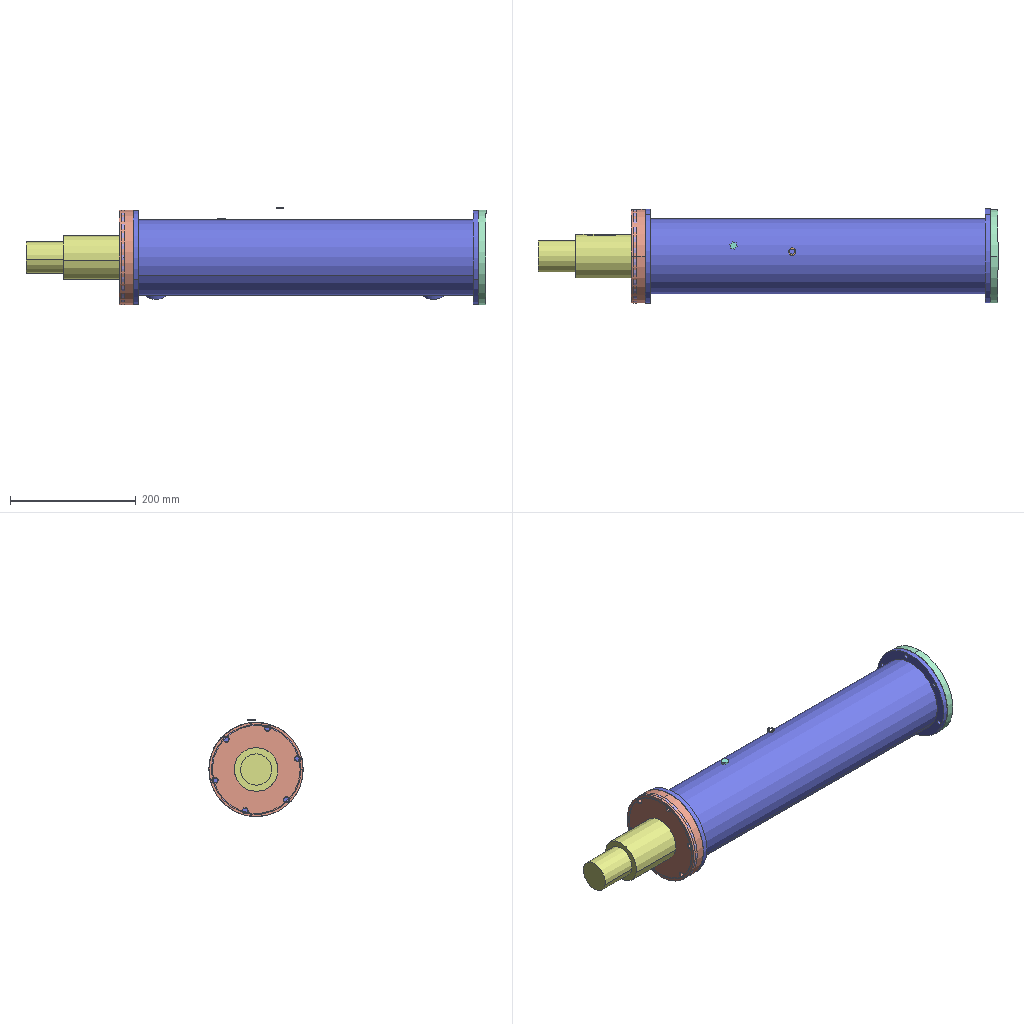Assembly | SolidWorks | 15 different items | 15 placed | box 733 x 151 x 155 mm
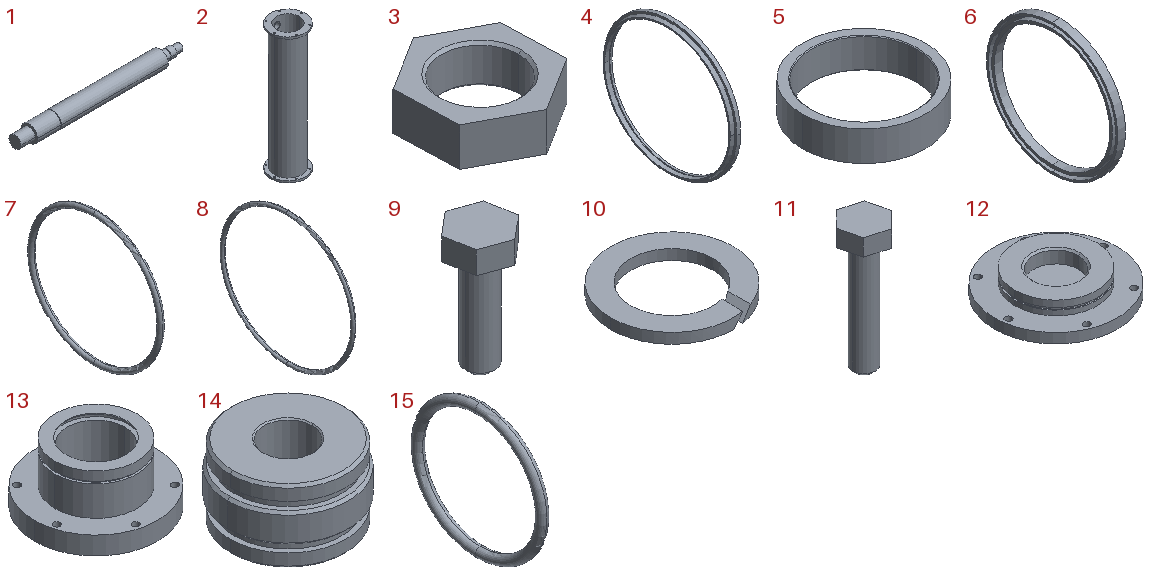Parts list (item | quantity | size | volume | features):
1 | x1 | 691.99 x 70 x 70 mm | 2315644 mm3 | features ICE 1, Revolution 1
2 | x1 | 150.705 x 150 x 550 mm | 1989302 mm3 | features ICE 6, Chamfer 1, Extrusion 1
3 | x1 | 44.157 x 49.969 x 15 mm | 13658 mm3 | features Chamfer 1, Extrusion 1
4 | x1 | 8.3 x 150 x 150 mm | 13389 mm3 | features Revolution 1
5 | x1 | 82 x 82 x 20 mm | 28596 mm3 | features Chamfer 1, Extrusion 1
6 | x1 | 6 x 100 x 100 mm | 7223 mm3 | features Revolution 1
7 | x1 | 2.65 x 67.35 x 67.35 mm | 1121 mm3 | features Revolution 1
8 | x1 | 2.65 x 97.35 x 97.35 mm | 1641 mm3 | features Revolution 1
9 | x1 | 11.292 x 11.809 x 24.5 mm | 977.997 mm3 | features ICE 2, Chamfer 1, Extrusion 1
10 | x1 | 12 x 12 x 1 mm | 60.867 mm3 | features Extrusion 1, ICE 1
11 | x1 | 11.534 x 11.645 x 34.5 mm | 1261 mm3 | features ICE 2, Chamfer 1, Extrusion 1
12 | x1 | 150 x 150 x 28.5 mm | 297244 mm3 | features ICE 5, Chamfer 1, Extrusion 1
13 | x1 | 150 x 150 x 72 mm | 489629 mm3 | features ICE 3, Chamfer 1, Extrusion 1, RevCut 1
14 | x1 | 100 x 100 x 60 mm | 356087 mm3 | features ICE 4, Chamfer 3, Extrusion 1
15 | x1 | 2.65 x 37.35 x 37.35 mm | 601.258 mm3 | features Revolution 1
Mates (type | each side: item.copy, entity, surface, feature):
Concentric | 12.1 edge | 2.1 edge
Concentric | 13.1 edge | 2.1 edge
Coincident | 12.1 face plane Boss-Extrude1 | 2.1 face plane Boss-Extrude1
Coincident | 13.1 face plane Boss-Extrude1 | 2.1 face plane Boss-Extrude1
Concentric | 6.1 edge | 14.1 edge
Concentric | 8.1 axis | 13.1 edge
Coincident | 1.1 face plane Revolve1 | 3.1 edge
Coincident | 1.1 face plane Revolve1 | 3.1 face plane Boss-Extrude1
Concentric | 1.1 edge | 3.1 edge
Parallel | 1.1 face plane Revolve1 | 13.1 face plane Boss-Extrude1
Concentric | 1.1 edge | 13.1 edge
Concentric | 14.1 edge | 2.1 edge
Parallel | 5.1 face plane Boss-Extrude1 | 13.1 face plane Boss-Extrude1
Concentric | 5.1 edge | 2.1 edge
Concentric | 4.1 edge | 13.1 edge